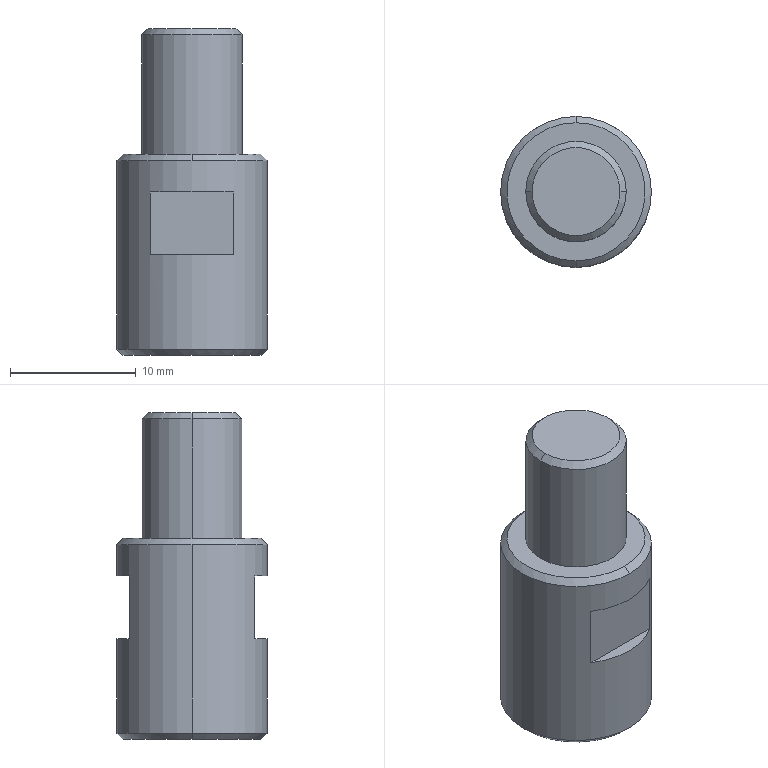Part | STEP file | PN_0019 Locating pin | 1 solid | 19 faces | box 12 x 12 x 26 mm | volume 2255 mm3 | plane 9 | cone 6 | cylinder 4 | commonest cylinder face diameters 8 x2 12 x2
STEP:
#1=CARTESIAN_POINT('',(0.,0.,0.));
#2=DIRECTION('',(0.,0.,1.));
#3=DIRECTION('',(1.,0.,0.));
#4=AXIS2_PLACEMENT_3D('',#1,#2,#3);
#5=CARTESIAN_POINT('',(-3.317,5.,8.));
#6=VERTEX_POINT('',#5);
#7=CARTESIAN_POINT('',(3.317,5.,8.));
#8=VERTEX_POINT('',#7);
#9=CARTESIAN_POINT('',(0.,0.,8.));
#10=DIRECTION('',(0.,0.,-1.));
#11=DIRECTION('',(-1.,0.,0.));
#12=AXIS2_PLACEMENT_3D('',#9,#10,#11);
#13=CIRCLE('',#12,6.);
#14=CARTESIAN_POINT('',(0.,0.,16.));
#15=DIRECTION('',(0.,0.,-1.));
#16=DIRECTION('',(-1.,0.,0.));
#17=AXIS2_PLACEMENT_3D('',#14,#15,#16);
#18=CYLINDRICAL_SURFACE('',#17,6.);
#19=CARTESIAN_POINT('',(0.,8.));
#20=DIRECTION('',(1.,0.));
#21=VECTOR('',#20,1.);
#22=LINE('',#19,#21);
#23=(GEOMETRIC_REPRESENTATION_CONTEXT(2)PARAMETRIC_REPRESENTATION_CONTEXT()REPRESENTATION_CONTEXT('',''));
#24=DEFINITIONAL_REPRESENTATION('',(#22),#23);
#25=PCURVE('',#18,#24);
#26=CARTESIAN_POINT('',(-6.,10.,8.));
#27=DIRECTION('',(0.,0.,-1.));
#28=DIRECTION('',(-1.,0.,0.));
#29=AXIS2_PLACEMENT_3D('',#26,#27,#28);
#30=PLANE('',#29);
#31=CARTESIAN_POINT('',(-6.,-10.));
#32=DIRECTION('',(1.,0.));
#33=AXIS2_PLACEMENT_2D('',#31,#32);
#34=CIRCLE('',#33,6.);
#35=(GEOMETRIC_REPRESENTATION_CONTEXT(2)PARAMETRIC_REPRESENTATION_CONTEXT()REPRESENTATION_CONTEXT('',''));
#36=DEFINITIONAL_REPRESENTATION('',(#34),#35);
#37=PCURVE('',#30,#36);
#38=SURFACE_CURVE('',#13,(#25,#37),.PCURVE_S1.);
#39=EDGE_CURVE('',#6,#8,#38,.T.);
#40=ORIENTED_EDGE('',*,*,#39,.T.);
#41=CARTESIAN_POINT('',(3.317,5.,13.));
#42=VERTEX_POINT('',#41);
#43=CARTESIAN_POINT('',(3.317,5.,16.));
#44=DIRECTION('',(0.,0.,1.));
#45=VECTOR('',#44,1.);
#46=LINE('',#43,#45);
#47=CARTESIAN_POINT('',(2.156,0.));
#48=DIRECTION('',(0.,-1.));
#49=VECTOR('',#48,1.);
#50=LINE('',#47,#49);
#51=(GEOMETRIC_REPRESENTATION_CONTEXT(2)PARAMETRIC_REPRESENTATION_CONTEXT()REPRESENTATION_CONTEXT('',''));
#52=DEFINITIONAL_REPRESENTATION('',(#50),#51);
#53=PCURVE('',#18,#52);
#54=CARTESIAN_POINT('',(-6.,5.,8.));
#55=DIRECTION('',(0.,-1.,0.));
#56=DIRECTION('',(0.,0.,-1.));
#57=AXIS2_PLACEMENT_3D('',#54,#55,#56);
#58=PLANE('',#57);
#59=CARTESIAN_POINT('',(-8.,9.317));
#60=DIRECTION('',(-1.,0.));
#61=VECTOR('',#60,1.);
#62=LINE('',#59,#61);
#63=(GEOMETRIC_REPRESENTATION_CONTEXT(2)PARAMETRIC_REPRESENTATION_CONTEXT()REPRESENTATION_CONTEXT('',''));
#64=DEFINITIONAL_REPRESENTATION('',(#62),#63);
#65=PCURVE('',#58,#64);
#66=SURFACE_CURVE('',#46,(#53,#65),.PCURVE_S1.);
#67=EDGE_CURVE('',#8,#42,#66,.T.);
#68=ORIENTED_EDGE('',*,*,#67,.T.);
#69=CARTESIAN_POINT('',(-3.317,5.,13.));
#70=VERTEX_POINT('',#69);
#71=CARTESIAN_POINT('',(0.,0.,13.));
#72=DIRECTION('',(0.,0.,1.));
#73=DIRECTION('',(-1.,0.,0.));
#74=AXIS2_PLACEMENT_3D('',#71,#72,#73);
#75=CIRCLE('',#74,6.);
#76=CARTESIAN_POINT('',(6.283,3.));
#77=DIRECTION('',(-1.,0.));
#78=VECTOR('',#77,1.);
#79=LINE('',#76,#78);
#80=(GEOMETRIC_REPRESENTATION_CONTEXT(2)PARAMETRIC_REPRESENTATION_CONTEXT()REPRESENTATION_CONTEXT('',''));
#81=DEFINITIONAL_REPRESENTATION('',(#79),#80);
#82=PCURVE('',#18,#81);
#83=CARTESIAN_POINT('',(-6.,10.,13.));
#84=DIRECTION('',(0.,0.,1.));
#85=DIRECTION('',(1.,0.,0.));
#86=AXIS2_PLACEMENT_3D('',#83,#84,#85);
#87=PLANE('',#86);
#88=CARTESIAN_POINT('',(6.,-10.));
#89=DIRECTION('',(-1.,0.));
#90=AXIS2_PLACEMENT_2D('',#88,#89);
#91=CIRCLE('',#90,6.);
#92=(GEOMETRIC_REPRESENTATION_CONTEXT(2)PARAMETRIC_REPRESENTATION_CONTEXT()REPRESENTATION_CONTEXT('',''));
#93=DEFINITIONAL_REPRESENTATION('',(#91),#92);
#94=PCURVE('',#87,#93);
#95=SURFACE_CURVE('',#75,(#82,#94),.PCURVE_S1.);
#96=EDGE_CURVE('',#42,#70,#95,.T.);
#97=ORIENTED_EDGE('',*,*,#96,.T.);
#98=CARTESIAN_POINT('',(-3.317,5.,16.));
#99=DIRECTION('',(0.,0.,-1.));
#100=VECTOR('',#99,1.);
#101=LINE('',#98,#100);
#102=CARTESIAN_POINT('',(0.9851,0.));
#103=DIRECTION('',(0.,1.));
#104=VECTOR('',#103,1.);
#105=LINE('',#102,#104);
#106=(GEOMETRIC_REPRESENTATION_CONTEXT(2)PARAMETRIC_REPRESENTATION_CONTEXT()REPRESENTATION_CONTEXT('',''));
#107=DEFINITIONAL_REPRESENTATION('',(#105),#106);
#108=PCURVE('',#18,#107);
#109=CARTESIAN_POINT('',(-8.,2.683));
#110=DIRECTION('',(1.,0.));
#111=VECTOR('',#110,1.);
#112=LINE('',#109,#111);
#113=(GEOMETRIC_REPRESENTATION_CONTEXT(2)PARAMETRIC_REPRESENTATION_CONTEXT()REPRESENTATION_CONTEXT('',''));
#114=DEFINITIONAL_REPRESENTATION('',(#112),#113);
#115=PCURVE('',#58,#114);
#116=SURFACE_CURVE('',#101,(#108,#115),.PCURVE_S1.);
#117=EDGE_CURVE('',#70,#6,#116,.T.);
#118=ORIENTED_EDGE('',*,*,#117,.T.);
#119=EDGE_LOOP('',(#40,#68,#97,#118));
#120=FACE_BOUND('',#119,.T.);
#121=CARTESIAN_POINT('',(0.,6.,15.5));
#122=VERTEX_POINT('',#121);
#123=CARTESIAN_POINT('',(6.,0.,15.5));
#124=VERTEX_POINT('',#123);
#125=CARTESIAN_POINT('',(0.,0.,15.5));
#126=DIRECTION('',(0.,0.,-1.));
#127=DIRECTION('',(-1.,0.,0.));
#128=AXIS2_PLACEMENT_3D('',#125,#126,#127);
#129=CIRCLE('',#128,6.);
#130=CARTESIAN_POINT('',(0.,0.5));
#131=DIRECTION('',(1.,0.));
#132=VECTOR('',#131,1.);
#133=LINE('',#130,#132);
#134=(GEOMETRIC_REPRESENTATION_CONTEXT(2)PARAMETRIC_REPRESENTATION_CONTEXT()REPRESENTATION_CONTEXT('',''));
#135=DEFINITIONAL_REPRESENTATION('',(#133),#134);
#136=PCURVE('',#18,#135);
#137=CARTESIAN_POINT('',(0.,0.,15.5));
#138=DIRECTION('',(0.,0.,-1.));
#139=DIRECTION('',(0.,1.,0.));
#140=AXIS2_PLACEMENT_3D('',#137,#138,#139);
#141=CONICAL_SURFACE('',#140,6.,0.7854);
#142=CARTESIAN_POINT('',(-1.571,0.));
#143=DIRECTION('',(1.,0.));
#144=VECTOR('',#143,1.);
#145=LINE('',#142,#144);
#146=(GEOMETRIC_REPRESENTATION_CONTEXT(2)PARAMETRIC_REPRESENTATION_CONTEXT()REPRESENTATION_CONTEXT('',''));
#147=DEFINITIONAL_REPRESENTATION('',(#145),#146);
#148=PCURVE('',#141,#147);
#149=SURFACE_CURVE('',#129,(#136,#148),.PCURVE_S1.);
#150=EDGE_CURVE('',#122,#124,#149,.T.);
#151=ORIENTED_EDGE('',*,*,#150,.T.);
#152=CARTESIAN_POINT('',(6.,0.,0.5));
#153=VERTEX_POINT('',#152);
#154=CARTESIAN_POINT('',(6.,0.,16.));
#155=DIRECTION('',(0.,0.,-1.));
#156=VECTOR('',#155,1.);
#157=LINE('',#154,#156);
#158=CARTESIAN_POINT('',(3.142,0.));
#159=DIRECTION('',(0.,1.));
#160=VECTOR('',#159,1.);
#161=LINE('',#158,#160);
#162=(GEOMETRIC_REPRESENTATION_CONTEXT(2)PARAMETRIC_REPRESENTATION_CONTEXT()REPRESENTATION_CONTEXT('',''));
#163=DEFINITIONAL_REPRESENTATION('',(#161),#162);
#164=PCURVE('',#18,#163);
#165=CARTESIAN_POINT('',(0.,0.,16.));
#166=DIRECTION('',(0.,0.,-1.));
#167=DIRECTION('',(-1.,0.,0.));
#168=AXIS2_PLACEMENT_3D('',#165,#166,#167);
#169=CYLINDRICAL_SURFACE('',#168,6.);
#170=CARTESIAN_POINT('',(3.142,0.));
#171=DIRECTION('',(0.,1.));
#172=VECTOR('',#171,1.);
#173=LINE('',#170,#172);
#174=(GEOMETRIC_REPRESENTATION_CONTEXT(2)PARAMETRIC_REPRESENTATION_CONTEXT()REPRESENTATION_CONTEXT('',''));
#175=DEFINITIONAL_REPRESENTATION('',(#173),#174);
#176=PCURVE('',#169,#175);
#177=SURFACE_CURVE('',#157,(#164,#176),.PCURVE_S1.);
#178=EDGE_CURVE('',#124,#153,#177,.T.);
#179=ORIENTED_EDGE('',*,*,#178,.T.);
#180=CARTESIAN_POINT('',(-6.,0.,0.5));
#181=VERTEX_POINT('',#180);
#182=CARTESIAN_POINT('',(0.,0.,0.5));
#183=DIRECTION('',(0.,0.,1.));
#184=DIRECTION('',(-1.,0.,0.));
#185=AXIS2_PLACEMENT_3D('',#182,#183,#184);
#186=CIRCLE('',#185,6.);
#187=CARTESIAN_POINT('',(6.283,15.5));
#188=DIRECTION('',(-1.,0.));
#189=VECTOR('',#188,1.);
#190=LINE('',#187,#189);
#191=(GEOMETRIC_REPRESENTATION_CONTEXT(2)PARAMETRIC_REPRESENTATION_CONTEXT()REPRESENTATION_CONTEXT('',''));
#192=DEFINITIONAL_REPRESENTATION('',(#190),#191);
#193=PCURVE('',#18,#192);
#194=CARTESIAN_POINT('',(0.,0.,0.5));
#195=DIRECTION('',(0.,0.,1.));
#196=DIRECTION('',(1.,0.,0.));
#197=AXIS2_PLACEMENT_3D('',#194,#195,#196);
#198=CONICAL_SURFACE('',#197,6.,0.7854);
#199=CARTESIAN_POINT('',(-3.142,0.));
#200=DIRECTION('',(1.,0.));
#201=VECTOR('',#200,1.);
#202=LINE('',#199,#201);
#203=(GEOMETRIC_REPRESENTATION_CONTEXT(2)PARAMETRIC_REPRESENTATION_CONTEXT()REPRESENTATION_CONTEXT('',''));
#204=DEFINITIONAL_REPRESENTATION('',(#202),#203);
#205=PCURVE('',#198,#204);
#206=SURFACE_CURVE('',#186,(#193,#205),.PCURVE_S1.);
#207=EDGE_CURVE('',#153,#181,#206,.T.);
#208=ORIENTED_EDGE('',*,*,#207,.T.);
#209=CARTESIAN_POINT('',(-6.,0.,15.5));
#210=VERTEX_POINT('',#209);
#211=CARTESIAN_POINT('',(-6.,0.,16.));
#212=DIRECTION('',(0.,0.,-1.));
#213=VECTOR('',#212,1.);
#214=LINE('',#211,#213);
#215=CARTESIAN_POINT('',(0.,0.));
#216=DIRECTION('',(0.,1.));
#217=VECTOR('',#216,1.);
#218=LINE('',#215,#217);
#219=(GEOMETRIC_REPRESENTATION_CONTEXT(2)PARAMETRIC_REPRESENTATION_CONTEXT()REPRESENTATION_CONTEXT('',''));
#220=DEFINITIONAL_REPRESENTATION('',(#218),#219);
#221=PCURVE('',#18,#220);
#222=CARTESIAN_POINT('',(6.283,0.));
#223=DIRECTION('',(0.,1.));
#224=VECTOR('',#223,1.);
#225=LINE('',#222,#224);
#226=(GEOMETRIC_REPRESENTATION_CONTEXT(2)PARAMETRIC_REPRESENTATION_CONTEXT()REPRESENTATION_CONTEXT('',''));
#227=DEFINITIONAL_REPRESENTATION('',(#225),#226);
#228=PCURVE('',#169,#227);
#229=SURFACE_CURVE('',#214,(#221,#228),.PCURVE_S1.);
#230=EDGE_CURVE('',#210,#181,#229,.T.);
#231=ORIENTED_EDGE('',*,*,#230,.F.);
#232=CARTESIAN_POINT('',(0.,0.,15.5));
#233=DIRECTION('',(0.,0.,-1.));
#234=DIRECTION('',(-1.,0.,0.));
#235=AXIS2_PLACEMENT_3D('',#232,#233,#234);
#236=CIRCLE('',#235,6.);
#237=CARTESIAN_POINT('',(0.,0.5));
#238=DIRECTION('',(1.,0.));
#239=VECTOR('',#238,1.);
#240=LINE('',#237,#239);
#241=(GEOMETRIC_REPRESENTATION_CONTEXT(2)PARAMETRIC_REPRESENTATION_CONTEXT()REPRESENTATION_CONTEXT('',''));
#242=DEFINITIONAL_REPRESENTATION('',(#240),#241);
#243=PCURVE('',#18,#242);
#244=CARTESIAN_POINT('',(0.,0.,15.5));
#245=DIRECTION('',(0.,0.,-1.));
#246=DIRECTION('',(0.,1.,0.));
#247=AXIS2_PLACEMENT_3D('',#244,#245,#246);
#248=CONICAL_SURFACE('',#247,6.,0.7854);
#249=CARTESIAN_POINT('',(4.712,0.));
#250=DIRECTION('',(1.,0.));
#251=VECTOR('',#250,1.);
#252=LINE('',#249,#251);
#253=(GEOMETRIC_REPRESENTATION_CONTEXT(2)PARAMETRIC_REPRESENTATION_CONTEXT()REPRESENTATION_CONTEXT('',''));
#254=DEFINITIONAL_REPRESENTATION('',(#252),#253);
#255=PCURVE('',#248,#254);
#256=SURFACE_CURVE('',#236,(#243,#255),.PCURVE_S1.);
#257=EDGE_CURVE('',#210,#122,#256,.T.);
#258=ORIENTED_EDGE('',*,*,#257,.T.);
#259=EDGE_LOOP('',(#151,#179,#208,#231,#258));
#260=FACE_BOUND('',#259,.T.);
#261=ADVANCED_FACE('',(#120,#260),#18,.T.);
#262=CARTESIAN_POINT('',(5.5,0.,0.));
#263=VERTEX_POINT('',#262);
#264=CARTESIAN_POINT('',(-5.5,0.,0.));
#265=VERTEX_POINT('',#264);
#266=CARTESIAN_POINT('',(0.,0.,0.));
#267=DIRECTION('',(0.,0.,1.));
#268=DIRECTION('',(1.,0.,0.));
#269=AXIS2_PLACEMENT_3D('',#266,#267,#268);
#270=CIRCLE('',#269,5.5);
#271=CARTESIAN_POINT('',(0.,-0.5));
#272=DIRECTION('',(1.,0.));
#273=VECTOR('',#272,1.);
#274=LINE('',#271,#273);
#275=(GEOMETRIC_REPRESENTATION_CONTEXT(2)PARAMETRIC_REPRESENTATION_CONTEXT()REPRESENTATION_CONTEXT('',''));
#276=DEFINITIONAL_REPRESENTATION('',(#274),#275);
#277=PCURVE('',#198,#276);
#278=CARTESIAN_POINT('',(0.,0.,0.));
#279=DIRECTION('',(0.,0.,1.));
#280=DIRECTION('',(1.,0.,0.));
#281=AXIS2_PLACEMENT_3D('',#278,#279,#280);
#282=PLANE('',#281);
#283=CARTESIAN_POINT('',(0.,0.));
#284=DIRECTION('',(1.,0.));
#285=AXIS2_PLACEMENT_2D('',#283,#284);
#286=CIRCLE('',#285,5.5);
#287=(GEOMETRIC_REPRESENTATION_CONTEXT(2)PARAMETRIC_REPRESENTATION_CONTEXT()REPRESENTATION_CONTEXT('',''));
#288=DEFINITIONAL_REPRESENTATION('',(#286),#287);
#289=PCURVE('',#282,#288);
#290=SURFACE_CURVE('',#270,(#277,#289),.PCURVE_S1.);
#291=EDGE_CURVE('',#263,#265,#290,.T.);
#292=ORIENTED_EDGE('',*,*,#291,.T.);
#293=CARTESIAN_POINT('',(-6.,0.,0.5));
#294=DIRECTION('',(-0.7071,0.,0.7071));
#295=VECTOR('',#294,1.);
#296=LINE('',#293,#295);
#297=CARTESIAN_POINT('',(3.142,0.));
#298=DIRECTION('',(0.,1.));
#299=VECTOR('',#298,1.);
#300=LINE('',#297,#299);
#301=(GEOMETRIC_REPRESENTATION_CONTEXT(2)PARAMETRIC_REPRESENTATION_CONTEXT()REPRESENTATION_CONTEXT('',''));
#302=DEFINITIONAL_REPRESENTATION('',(#300),#301);
#303=PCURVE('',#198,#302);
#304=CARTESIAN_POINT('',(0.,0.,0.5));
#305=DIRECTION('',(0.,0.,1.));
#306=DIRECTION('',(1.,0.,0.));
#307=AXIS2_PLACEMENT_3D('',#304,#305,#306);
#308=CONICAL_SURFACE('',#307,6.,0.7854);
#309=CARTESIAN_POINT('',(3.142,0.));
#310=DIRECTION('',(0.,1.));
#311=VECTOR('',#310,1.);
#312=LINE('',#309,#311);
#313=(GEOMETRIC_REPRESENTATION_CONTEXT(2)PARAMETRIC_REPRESENTATION_CONTEXT()REPRESENTATION_CONTEXT('',''));
#314=DEFINITIONAL_REPRESENTATION('',(#312),#313);
#315=PCURVE('',#308,#314);
#316=SURFACE_CURVE('',#296,(#303,#315),.PCURVE_S1.);
#317=EDGE_CURVE('',#265,#181,#316,.T.);
#318=ORIENTED_EDGE('',*,*,#317,.T.);
#319=ORIENTED_EDGE('',*,*,#207,.F.);
#320=CARTESIAN_POINT('',(6.,0.,0.5));
#321=DIRECTION('',(0.7071,0.,0.7071));
#322=VECTOR('',#321,1.);
#323=LINE('',#320,#322);
#324=CARTESIAN_POINT('',(0.,0.));
#325=DIRECTION('',(0.,1.));
#326=VECTOR('',#325,1.);
#327=LINE('',#324,#326);
#328=(GEOMETRIC_REPRESENTATION_CONTEXT(2)PARAMETRIC_REPRESENTATION_CONTEXT()REPRESENTATION_CONTEXT('',''));
#329=DEFINITIONAL_REPRESENTATION('',(#327),#328);
#330=PCURVE('',#198,#329);
#331=CARTESIAN_POINT('',(6.283,0.));
#332=DIRECTION('',(0.,1.));
#333=VECTOR('',#332,1.);
#334=LINE('',#331,#333);
#335=(GEOMETRIC_REPRESENTATION_CONTEXT(2)PARAMETRIC_REPRESENTATION_CONTEXT()REPRESENTATION_CONTEXT('',''));
#336=DEFINITIONAL_REPRESENTATION('',(#334),#335);
#337=PCURVE('',#308,#336);
#338=SURFACE_CURVE('',#323,(#330,#337),.PCURVE_S1.);
#339=EDGE_CURVE('',#263,#153,#338,.T.);
#340=ORIENTED_EDGE('',*,*,#339,.F.);
#341=EDGE_LOOP('',(#292,#318,#319,#340));
#342=FACE_BOUND('',#341,.T.);
#343=ADVANCED_FACE('',(#342),#198,.T.);
#344=CARTESIAN_POINT('',(0.,5.5,16.));
#345=VERTEX_POINT('',#344);
#346=CARTESIAN_POINT('',(0.,-5.5,16.));
#347=VERTEX_POINT('',#346);
#348=CARTESIAN_POINT('',(0.,0.,16.));
#349=DIRECTION('',(0.,0.,-1.));
#350=DIRECTION('',(0.,1.,0.));
#351=AXIS2_PLACEMENT_3D('',#348,#349,#350);
#352=CIRCLE('',#351,5.5);
#353=CARTESIAN_POINT('',(0.,-0.5));
#354=DIRECTION('',(1.,0.));
#355=VECTOR('',#354,1.);
#356=LINE('',#353,#355);
#357=(GEOMETRIC_REPRESENTATION_CONTEXT(2)PARAMETRIC_REPRESENTATION_CONTEXT()REPRESENTATION_CONTEXT('',''));
#358=DEFINITIONAL_REPRESENTATION('',(#356),#357);
#359=PCURVE('',#141,#358);
#360=CARTESIAN_POINT('',(0.,0.,16.));
#361=DIRECTION('',(0.,0.,1.));
#362=DIRECTION('',(1.,0.,0.));
#363=AXIS2_PLACEMENT_3D('',#360,#361,#362);
#364=PLANE('',#363);
#365=CARTESIAN_POINT('',(0.,5.5));
#366=CARTESIAN_POINT('',(9.526,5.5));
#367=CARTESIAN_POINT('',(4.763,-2.75));
#368=CARTESIAN_POINT('',(0.,-11.));
#369=CARTESIAN_POINT('',(-4.763,-2.75));
#370=CARTESIAN_POINT('',(-9.526,5.5));
#371=CARTESIAN_POINT('',(0.,5.5));
#372=(BOUNDED_CURVE()B_SPLINE_CURVE(2,(#365,#366,#367,#368,#369,#370,#371),.UNSPECIFIED.,.T.,.F.)B_SPLINE_CURVE_WITH_KNOTS((1,2,2,2,2,1),(-2.094,0.,2.094,4.189,6.283,8.378),.UNSPECIFIED.)CURVE()GEOMETRIC_REPRESENTATION_ITEM()RATIONAL_B_SPLINE_CURVE((1.,0.5,1.,0.5,1.,0.5,1.))REPRESENTATION_ITEM(''));
#373=(GEOMETRIC_REPRESENTATION_CONTEXT(2)PARAMETRIC_REPRESENTATION_CONTEXT()REPRESENTATION_CONTEXT('',''));
#374=DEFINITIONAL_REPRESENTATION('',(#372),#373);
#375=PCURVE('',#364,#374);
#376=SURFACE_CURVE('',#352,(#359,#375),.PCURVE_S1.);
#377=EDGE_CURVE('',#345,#347,#376,.T.);
#378=ORIENTED_EDGE('',*,*,#377,.T.);
#379=CARTESIAN_POINT('',(0.,-6.,15.5));
#380=VERTEX_POINT('',#379);
#381=CARTESIAN_POINT('',(0.,-6.,15.5));
#382=DIRECTION('',(0.,-0.7071,-0.7071));
#383=VECTOR('',#382,1.);
#384=LINE('',#381,#383);
#385=CARTESIAN_POINT('',(3.142,0.));
#386=DIRECTION('',(0.,1.));
#387=VECTOR('',#386,1.);
#388=LINE('',#385,#387);
#389=(GEOMETRIC_REPRESENTATION_CONTEXT(2)PARAMETRIC_REPRESENTATION_CONTEXT()REPRESENTATION_CONTEXT('',''));
#390=DEFINITIONAL_REPRESENTATION('',(#388),#389);
#391=PCURVE('',#141,#390);
#392=CARTESIAN_POINT('',(3.142,0.));
#393=DIRECTION('',(0.,1.));
#394=VECTOR('',#393,1.);
#395=LINE('',#392,#394);
#396=(GEOMETRIC_REPRESENTATION_CONTEXT(2)PARAMETRIC_REPRESENTATION_CONTEXT()REPRESENTATION_CONTEXT('',''));
#397=DEFINITIONAL_REPRESENTATION('',(#395),#396);
#398=PCURVE('',#248,#397);
#399=SURFACE_CURVE('',#384,(#391,#398),.PCURVE_S1.);
#400=EDGE_CURVE('',#347,#380,#399,.T.);
#401=ORIENTED_EDGE('',*,*,#400,.T.);
#402=CARTESIAN_POINT('',(0.,0.,15.5));
#403=DIRECTION('',(0.,0.,-1.));
#404=DIRECTION('',(-1.,0.,0.));
#405=AXIS2_PLACEMENT_3D('',#402,#403,#404);
#406=CIRCLE('',#405,6.);
#407=CARTESIAN_POINT('',(-1.571,0.));
#408=DIRECTION('',(1.,0.));
#409=VECTOR('',#408,1.);
#410=LINE('',#407,#409);
#411=(GEOMETRIC_REPRESENTATION_CONTEXT(2)PARAMETRIC_REPRESENTATION_CONTEXT()REPRESENTATION_CONTEXT('',''));
#412=DEFINITIONAL_REPRESENTATION('',(#410),#411);
#413=PCURVE('',#141,#412);
#414=CARTESIAN_POINT('',(0.,0.5));
#415=DIRECTION('',(1.,0.));
#416=VECTOR('',#415,1.);
#417=LINE('',#414,#416);
#418=(GEOMETRIC_REPRESENTATION_CONTEXT(2)PARAMETRIC_REPRESENTATION_CONTEXT()REPRESENTATION_CONTEXT('',''));
#419=DEFINITIONAL_REPRESENTATION('',(#417),#418);
#420=PCURVE('',#169,#419);
#421=SURFACE_CURVE('',#406,(#413,#420),.PCURVE_S1.);
#422=EDGE_CURVE('',#124,#380,#421,.T.);
#423=ORIENTED_EDGE('',*,*,#422,.F.);
#424=ORIENTED_EDGE('',*,*,#150,.F.);
#425=CARTESIAN_POINT('',(0.,6.,15.5));
#426=DIRECTION('',(0.,0.7071,-0.7071));
#427=VECTOR('',#426,1.);
#428=LINE('',#425,#427);
#429=CARTESIAN_POINT('',(0.,0.));
#430=DIRECTION('',(0.,1.));
#431=VECTOR('',#430,1.);
#432=LINE('',#429,#431);
#433=(GEOMETRIC_REPRESENTATION_CONTEXT(2)PARAMETRIC_REPRESENTATION_CONTEXT()REPRESENTATION_CONTEXT('',''));
#434=DEFINITIONAL_REPRESENTATION('',(#432),#433);
#435=PCURVE('',#141,#434);
#436=CARTESIAN_POINT('',(6.283,0.));
#437=DIRECTION('',(0.,1.));
#438=VECTOR('',#437,1.);
#439=LINE('',#436,#438);
#440=(GEOMETRIC_REPRESENTATION_CONTEXT(2)PARAMETRIC_REPRESENTATION_CONTEXT()REPRESENTATION_CONTEXT('',''));
#441=DEFINITIONAL_REPRESENTATION('',(#439),#440);
#442=PCURVE('',#248,#441);
#443=SURFACE_CURVE('',#428,(#435,#442),.PCURVE_S1.);
#444=EDGE_CURVE('',#345,#122,#443,.T.);
#445=ORIENTED_EDGE('',*,*,#444,.F.);
#446=EDGE_LOOP('',(#378,#401,#423,#424,#445));
#447=FACE_BOUND('',#446,.T.);
#448=ADVANCED_FACE('',(#447),#141,.T.);
#449=CARTESIAN_POINT('',(-4.,0.,25.5));
#450=VERTEX_POINT('',#449);
#451=CARTESIAN_POINT('',(4.,0.,25.5));
#452=VERTEX_POINT('',#451);
#453=CARTESIAN_POINT('',(0.,0.,25.5));
#454=DIRECTION('',(0.,0.,-1.));
#455=DIRECTION('',(-1.,0.,0.));
#456=AXIS2_PLACEMENT_3D('',#453,#454,#455);
#457=CIRCLE('',#456,4.);
#458=CARTESIAN_POINT('',(0.,0.,26.));
#459=DIRECTION('',(0.,0.,-1.));
#460=DIRECTION('',(-1.,0.,0.));
#461=AXIS2_PLACEMENT_3D('',#458,#459,#460);
#462=CYLINDRICAL_SURFACE('',#461,4.);
#463=CARTESIAN_POINT('',(0.,0.5));
#464=DIRECTION('',(1.,0.));
#465=VECTOR('',#464,1.);
#466=LINE('',#463,#465);
#467=(GEOMETRIC_REPRESENTATION_CONTEXT(2)PARAMETRIC_REPRESENTATION_CONTEXT()REPRESENTATION_CONTEXT('',''));
#468=DEFINITIONAL_REPRESENTATION('',(#466),#467);
#469=PCURVE('',#462,#468);
#470=CARTESIAN_POINT('',(0.,0.,25.5));
#471=DIRECTION('',(0.,0.,-1.));
#472=DIRECTION('',(-1.,0.,0.));
#473=AXIS2_PLACEMENT_3D('',#470,#471,#472);
#474=CONICAL_SURFACE('',#473,4.,0.7854);
#475=CARTESIAN_POINT('',(0.,0.));
#476=DIRECTION('',(1.,0.));
#477=VECTOR('',#476,1.);
#478=LINE('',#475,#477);
#479=(GEOMETRIC_REPRESENTATION_CONTEXT(2)PARAMETRIC_REPRESENTATION_CONTEXT()REPRESENTATION_CONTEXT('',''));
#480=DEFINITIONAL_REPRESENTATION('',(#478),#479);
#481=PCURVE('',#474,#480);
#482=SURFACE_CURVE('',#457,(#469,#481),.PCURVE_S1.);
#483=EDGE_CURVE('',#450,#452,#482,.T.);
#484=ORIENTED_EDGE('',*,*,#483,.T.);
#485=CARTESIAN_POINT('',(4.,0.,16.));
#486=VERTEX_POINT('',#485);
#487=CARTESIAN_POINT('',(4.,0.,26.));
#488=DIRECTION('',(0.,0.,-1.));
#489=VECTOR('',#488,1.);
#490=LINE('',#487,#489);
#491=CARTESIAN_POINT('',(3.142,0.));
#492=DIRECTION('',(0.,1.));
#493=VECTOR('',#492,1.);
#494=LINE('',#491,#493);
#495=(GEOMETRIC_REPRESENTATION_CONTEXT(2)PARAMETRIC_REPRESENTATION_CONTEXT()REPRESENTATION_CONTEXT('',''));
#496=DEFINITIONAL_REPRESENTATION('',(#494),#495);
#497=PCURVE('',#462,#496);
#498=CARTESIAN_POINT('',(0.,0.,26.));
#499=DIRECTION('',(0.,0.,-1.));
#500=DIRECTION('',(-1.,0.,0.));
#501=AXIS2_PLACEMENT_3D('',#498,#499,#500);
#502=CYLINDRICAL_SURFACE('',#501,4.);
#503=CARTESIAN_POINT('',(3.142,0.));
#504=DIRECTION('',(0.,1.));
#505=VECTOR('',#504,1.);
#506=LINE('',#503,#505);
#507=(GEOMETRIC_REPRESENTATION_CONTEXT(2)PARAMETRIC_REPRESENTATION_CONTEXT()REPRESENTATION_CONTEXT('',''));
#508=DEFINITIONAL_REPRESENTATION('',(#506),#507);
#509=PCURVE('',#502,#508);
#510=SURFACE_CURVE('',#490,(#497,#509),.PCURVE_S1.);
#511=EDGE_CURVE('',#452,#486,#510,.T.);
#512=ORIENTED_EDGE('',*,*,#511,.T.);
#513=CARTESIAN_POINT('',(-4.,0.,16.));
#514=VERTEX_POINT('',#513);
#515=CARTESIAN_POINT('',(0.,0.,16.));
#516=DIRECTION('',(0.,0.,-1.));
#517=DIRECTION('',(-1.,0.,0.));
#518=AXIS2_PLACEMENT_3D('',#515,#516,#517);
#519=CIRCLE('',#518,4.);
#520=CARTESIAN_POINT('',(0.,10.));
#521=DIRECTION('',(1.,0.));
#522=VECTOR('',#521,1.);
#523=LINE('',#520,#522);
#524=(GEOMETRIC_REPRESENTATION_CONTEXT(2)PARAMETRIC_REPRESENTATION_CONTEXT()REPRESENTATION_CONTEXT('',''));
#525=DEFINITIONAL_REPRESENTATION('',(#523),#524);
#526=PCURVE('',#462,#525);
#527=CARTESIAN_POINT('',(-4.,0.));
#528=CARTESIAN_POINT('',(-4.,6.928));
#529=CARTESIAN_POINT('',(2.,3.464));
#530=CARTESIAN_POINT('',(8.,0.));
#531=CARTESIAN_POINT('',(2.,-3.464));
#532=CARTESIAN_POINT('',(-4.,-6.928));
#533=CARTESIAN_POINT('',(-4.,0.));
#534=(BOUNDED_CURVE()B_SPLINE_CURVE(2,(#527,#528,#529,#530,#531,#532,#533),.UNSPECIFIED.,.T.,.F.)B_SPLINE_CURVE_WITH_KNOTS((1,2,2,2,2,1),(-2.094,0.,2.094,4.189,6.283,8.378),.UNSPECIFIED.)CURVE()GEOMETRIC_REPRESENTATION_ITEM()RATIONAL_B_SPLINE_CURVE((1.,0.5,1.,0.5,1.,0.5,1.))REPRESENTATION_ITEM(''));
#535=(GEOMETRIC_REPRESENTATION_CONTEXT(2)PARAMETRIC_REPRESENTATION_CONTEXT()REPRESENTATION_CONTEXT('',''));
#536=DEFINITIONAL_REPRESENTATION('',(#534),#535);
#537=PCURVE('',#364,#536);
#538=SURFACE_CURVE('',#519,(#526,#537),.PCURVE_S1.);
#539=EDGE_CURVE('',#514,#486,#538,.T.);
#540=ORIENTED_EDGE('',*,*,#539,.F.);
#541=CARTESIAN_POINT('',(-4.,0.,26.));
#542=DIRECTION('',(0.,0.,-1.));
#543=VECTOR('',#542,1.);
#544=LINE('',#541,#543);
#545=CARTESIAN_POINT('',(0.,0.));
#546=DIRECTION('',(0.,1.));
#547=VECTOR('',#546,1.);
#548=LINE('',#545,#547);
#549=(GEOMETRIC_REPRESENTATION_CONTEXT(2)PARAMETRIC_REPRESENTATION_CONTEXT()REPRESENTATION_CONTEXT('',''));
#550=DEFINITIONAL_REPRESENTATION('',(#548),#549);
#551=PCURVE('',#462,#550);
#552=CARTESIAN_POINT('',(6.283,0.));
#553=DIRECTION('',(0.,1.));
#554=VECTOR('',#553,1.);
#555=LINE('',#552,#554);
#556=(GEOMETRIC_REPRESENTATION_CONTEXT(2)PARAMETRIC_REPRESENTATION_CONTEXT()REPRESENTATION_CONTEXT('',''));
#557=DEFINITIONAL_REPRESENTATION('',(#555),#556);
#558=PCURVE('',#502,#557);
#559=SURFACE_CURVE('',#544,(#551,#558),.PCURVE_S1.);
#560=EDGE_CURVE('',#450,#514,#559,.T.);
#561=ORIENTED_EDGE('',*,*,#560,.F.);
#562=EDGE_LOOP('',(#484,#512,#540,#561));
#563=FACE_BOUND('',#562,.T.);
#564=ADVANCED_FACE('',(#563),#462,.T.);
#565=CARTESIAN_POINT('',(-3.5,0.,26.));
#566=VERTEX_POINT('',#565);
#567=CARTESIAN_POINT('',(3.5,0.,26.));
#568=VERTEX_POINT('',#567);
#569=CARTESIAN_POINT('',(0.,0.,26.));
#570=DIRECTION('',(0.,0.,-1.));
#571=DIRECTION('',(-1.,0.,0.));
#572=AXIS2_PLACEMENT_3D('',#569,#570,#571);
#573=CIRCLE('',#572,3.5);
#574=CARTESIAN_POINT('',(0.,-0.5));
#575=DIRECTION('',(1.,0.));
#576=VECTOR('',#575,1.);
#577=LINE('',#574,#576);
#578=(GEOMETRIC_REPRESENTATION_CONTEXT(2)PARAMETRIC_REPRESENTATION_CONTEXT()REPRESENTATION_CONTEXT('',''));
#579=DEFINITIONAL_REPRESENTATION('',(#577),#578);
#580=PCURVE('',#474,#579);
#581=CARTESIAN_POINT('',(0.,0.,26.));
#582=DIRECTION('',(0.,0.,1.));
#583=DIRECTION('',(1.,0.,0.));
#584=AXIS2_PLACEMENT_3D('',#581,#582,#583);
#585=PLANE('',#584);
#586=CARTESIAN_POINT('',(-3.5,0.));
#587=CARTESIAN_POINT('',(-3.5,6.062));
#588=CARTESIAN_POINT('',(1.75,3.031));
#589=CARTESIAN_POINT('',(7.,0.));
#590=CARTESIAN_POINT('',(1.75,-3.031));
#591=CARTESIAN_POINT('',(-3.5,-6.062));
#592=CARTESIAN_POINT('',(-3.5,0.));
#593=(BOUNDED_CURVE()B_SPLINE_CURVE(2,(#586,#587,#588,#589,#590,#591,#592),.UNSPECIFIED.,.T.,.F.)B_SPLINE_CURVE_WITH_KNOTS((1,2,2,2,2,1),(-2.094,0.,2.094,4.189,6.283,8.378),.UNSPECIFIED.)CURVE()GEOMETRIC_REPRESENTATION_ITEM()RATIONAL_B_SPLINE_CURVE((1.,0.5,1.,0.5,1.,0.5,1.))REPRESENTATION_ITEM(''));
#594=(GEOMETRIC_REPRESENTATION_CONTEXT(2)PARAMETRIC_REPRESENTATION_CONTEXT()REPRESENTATION_CONTEXT('',''));
#595=DEFINITIONAL_REPRESENTATION('',(#593),#594);
#596=PCURVE('',#585,#595);
#597=SURFACE_CURVE('',#573,(#580,#596),.PCURVE_S1.);
#598=EDGE_CURVE('',#566,#568,#597,.T.);
#599=ORIENTED_EDGE('',*,*,#598,.T.);
#600=CARTESIAN_POINT('',(4.,0.,25.5));
#601=DIRECTION('',(0.7071,0.,-0.7071));
#602=VECTOR('',#601,1.);
#603=LINE('',#600,#602);
#604=CARTESIAN_POINT('',(3.142,0.));
#605=DIRECTION('',(0.,1.));
#606=VECTOR('',#605,1.);
#607=LINE('',#604,#606);
#608=(GEOMETRIC_REPRESENTATION_CONTEXT(2)PARAMETRIC_REPRESENTATION_CONTEXT()REPRESENTATION_CONTEXT('',''));
#609=DEFINITIONAL_REPRESENTATION('',(#607),#608);
#610=PCURVE('',#474,#609);
#611=CARTESIAN_POINT('',(0.,0.,25.5));
#612=DIRECTION('',(0.,0.,-1.));
#613=DIRECTION('',(-1.,0.,0.));
#614=AXIS2_PLACEMENT_3D('',#611,#612,#613);
#615=CONICAL_SURFACE('',#614,4.,0.7854);
#616=CARTESIAN_POINT('',(3.142,0.));
#617=DIRECTION('',(0.,1.));
#618=VECTOR('',#617,1.);
#619=LINE('',#616,#618);
#620=(GEOMETRIC_REPRESENTATION_CONTEXT(2)PARAMETRIC_REPRESENTATION_CONTEXT()REPRESENTATION_CONTEXT('',''));
#621=DEFINITIONAL_REPRESENTATION('',(#619),#620);
#622=PCURVE('',#615,#621);
#623=SURFACE_CURVE('',#603,(#610,#622),.PCURVE_S1.);
#624=EDGE_CURVE('',#568,#452,#623,.T.);
#625=ORIENTED_EDGE('',*,*,#624,.T.);
#626=ORIENTED_EDGE('',*,*,#483,.F.);
#627=CARTESIAN_POINT('',(-4.,0.,25.5));
#628=DIRECTION('',(-0.7071,0.,-0.7071));
#629=VECTOR('',#628,1.);
#630=LINE('',#627,#629);
#631=CARTESIAN_POINT('',(0.,0.));
#632=DIRECTION('',(0.,1.));
#633=VECTOR('',#632,1.);
#634=LINE('',#631,#633);
#635=(GEOMETRIC_REPRESENTATION_CONTEXT(2)PARAMETRIC_REPRESENTATION_CONTEXT()REPRESENTATION_CONTEXT('',''));
#636=DEFINITIONAL_REPRESENTATION('',(#634),#635);
#637=PCURVE('',#474,#636);
#638=CARTESIAN_POINT('',(6.283,0.));
#639=DIRECTION('',(0.,1.));
#640=VECTOR('',#639,1.);
#641=LINE('',#638,#640);
#642=(GEOMETRIC_REPRESENTATION_CONTEXT(2)PARAMETRIC_REPRESENTATION_CONTEXT()REPRESENTATION_CONTEXT('',''));
#643=DEFINITIONAL_REPRESENTATION('',(#641),#642);
#644=PCURVE('',#615,#643);
#645=SURFACE_CURVE('',#630,(#637,#644),.PCURVE_S1.);
#646=EDGE_CURVE('',#566,#450,#645,.T.);
#647=ORIENTED_EDGE('',*,*,#646,.F.);
#648=EDGE_LOOP('',(#599,#625,#626,#647));
#649=FACE_BOUND('',#648,.T.);
#650=ADVANCED_FACE('',(#649),#474,.T.);
#651=ORIENTED_EDGE('',*,*,#178,.F.);
#652=ORIENTED_EDGE('',*,*,#422,.T.);
#653=CARTESIAN_POINT('',(0.,0.,15.5));
#654=DIRECTION('',(0.,0.,-1.));
#655=DIRECTION('',(-1.,0.,0.));
#656=AXIS2_PLACEMENT_3D('',#653,#654,#655);
#657=CIRCLE('',#656,6.);
#658=CARTESIAN_POINT('',(0.,0.5));
#659=DIRECTION('',(1.,0.));
#660=VECTOR('',#659,1.);
#661=LINE('',#658,#660);
#662=(GEOMETRIC_REPRESENTATION_CONTEXT(2)PARAMETRIC_REPRESENTATION_CONTEXT()REPRESENTATION_CONTEXT('',''));
#663=DEFINITIONAL_REPRESENTATION('',(#661),#662);
#664=PCURVE('',#169,#663);
#665=CARTESIAN_POINT('',(-1.571,0.));
#666=DIRECTION('',(1.,0.));
#667=VECTOR('',#666,1.);
#668=LINE('',#665,#667);
#669=(GEOMETRIC_REPRESENTATION_CONTEXT(2)PARAMETRIC_REPRESENTATION_CONTEXT()REPRESENTATION_CONTEXT('',''));
#670=DEFINITIONAL_REPRESENTATION('',(#668),#669);
#671=PCURVE('',#248,#670);
#672=SURFACE_CURVE('',#657,(#664,#671),.PCURVE_S1.);
#673=EDGE_CURVE('',#380,#210,#672,.T.);
#674=ORIENTED_EDGE('',*,*,#673,.T.);
#675=ORIENTED_EDGE('',*,*,#230,.T.);
#676=CARTESIAN_POINT('',(0.,0.,0.5));
#677=DIRECTION('',(0.,0.,1.));
#678=DIRECTION('',(-1.,0.,0.));
#679=AXIS2_PLACEMENT_3D('',#676,#677,#678);
#680=CIRCLE('',#679,6.);
#681=CARTESIAN_POINT('',(6.283,15.5));
#682=DIRECTION('',(-1.,0.));
#683=VECTOR('',#682,1.);
#684=LINE('',#681,#683);
#685=(GEOMETRIC_REPRESENTATION_CONTEXT(2)PARAMETRIC_REPRESENTATION_CONTEXT()REPRESENTATION_CONTEXT('',''));
#686=DEFINITIONAL_REPRESENTATION('',(#684),#685);
#687=PCURVE('',#169,#686);
#688=CARTESIAN_POINT('',(3.142,0.));
#689=DIRECTION('',(1.,0.));
#690=VECTOR('',#689,1.);
#691=LINE('',#688,#690);
#692=(GEOMETRIC_REPRESENTATION_CONTEXT(2)PARAMETRIC_REPRESENTATION_CONTEXT()REPRESENTATION_CONTEXT('',''));
#693=DEFINITIONAL_REPRESENTATION('',(#691),#692);
#694=PCURVE('',#308,#693);
#695=SURFACE_CURVE('',#680,(#687,#694),.PCURVE_S1.);
#696=EDGE_CURVE('',#181,#153,#695,.T.);
#697=ORIENTED_EDGE('',*,*,#696,.T.);
#698=EDGE_LOOP('',(#651,#652,#674,#675,#697));
#699=FACE_BOUND('',#698,.T.);
#700=CARTESIAN_POINT('',(3.317,-5.,8.));
#701=VERTEX_POINT('',#700);
#702=CARTESIAN_POINT('',(-3.317,-5.,8.));
#703=VERTEX_POINT('',#702);
#704=CARTESIAN_POINT('',(0.,0.,8.));
#705=DIRECTION('',(0.,0.,-1.));
#706=DIRECTION('',(-1.,0.,0.));
#707=AXIS2_PLACEMENT_3D('',#704,#705,#706);
#708=CIRCLE('',#707,6.);
#709=CARTESIAN_POINT('',(0.,8.));
#710=DIRECTION('',(1.,0.));
#711=VECTOR('',#710,1.);
#712=LINE('',#709,#711);
#713=(GEOMETRIC_REPRESENTATION_CONTEXT(2)PARAMETRIC_REPRESENTATION_CONTEXT()REPRESENTATION_CONTEXT('',''));
#714=DEFINITIONAL_REPRESENTATION('',(#712),#713);
#715=PCURVE('',#169,#714);
#716=CARTESIAN_POINT('',(-6.,-5.,8.));
#717=DIRECTION('',(0.,0.,-1.));
#718=DIRECTION('',(0.,1.,0.));
#719=AXIS2_PLACEMENT_3D('',#716,#717,#718);
#720=PLANE('',#719);
#721=CARTESIAN_POINT('',(5.,6.));
#722=DIRECTION('',(0.,-1.));
#723=AXIS2_PLACEMENT_2D('',#721,#722);
#724=CIRCLE('',#723,6.);
#725=(GEOMETRIC_REPRESENTATION_CONTEXT(2)PARAMETRIC_REPRESENTATION_CONTEXT()REPRESENTATION_CONTEXT('',''));
#726=DEFINITIONAL_REPRESENTATION('',(#724),#725);
#727=PCURVE('',#720,#726);
#728=SURFACE_CURVE('',#708,(#715,#727),.PCURVE_S1.);
#729=EDGE_CURVE('',#701,#703,#728,.T.);
#730=ORIENTED_EDGE('',*,*,#729,.T.);
#731=CARTESIAN_POINT('',(-3.317,-5.,13.));
#732=VERTEX_POINT('',#731);
#733=CARTESIAN_POINT('',(-3.317,-5.,16.));
#734=DIRECTION('',(0.,0.,1.));
#735=VECTOR('',#734,1.);
#736=LINE('',#733,#735);
#737=CARTESIAN_POINT('',(5.298,0.));
#738=DIRECTION('',(0.,-1.));
#739=VECTOR('',#738,1.);
#740=LINE('',#737,#739);
#741=(GEOMETRIC_REPRESENTATION_CONTEXT(2)PARAMETRIC_REPRESENTATION_CONTEXT()REPRESENTATION_CONTEXT('',''));
#742=DEFINITIONAL_REPRESENTATION('',(#740),#741);
#743=PCURVE('',#169,#742);
#744=CARTESIAN_POINT('',(-6.,-5.,8.));
#745=DIRECTION('',(0.,1.,0.));
#746=DIRECTION('',(0.,0.,1.));
#747=AXIS2_PLACEMENT_3D('',#744,#745,#746);
#748=PLANE('',#747);
#749=CARTESIAN_POINT('',(8.,2.683));
#750=DIRECTION('',(1.,0.));
#751=VECTOR('',#750,1.);
#752=LINE('',#749,#751);
#753=(GEOMETRIC_REPRESENTATION_CONTEXT(2)PARAMETRIC_REPRESENTATION_CONTEXT()REPRESENTATION_CONTEXT('',''));
#754=DEFINITIONAL_REPRESENTATION('',(#752),#753);
#755=PCURVE('',#748,#754);
#756=SURFACE_CURVE('',#736,(#743,#755),.PCURVE_S1.);
#757=EDGE_CURVE('',#703,#732,#756,.T.);
#758=ORIENTED_EDGE('',*,*,#757,.T.);
#759=CARTESIAN_POINT('',(3.317,-5.,13.));
#760=VERTEX_POINT('',#759);
#761=CARTESIAN_POINT('',(0.,0.,13.));
#762=DIRECTION('',(0.,0.,1.));
#763=DIRECTION('',(-1.,0.,0.));
#764=AXIS2_PLACEMENT_3D('',#761,#762,#763);
#765=CIRCLE('',#764,6.);
#766=CARTESIAN_POINT('',(6.283,3.));
#767=DIRECTION('',(-1.,0.));
#768=VECTOR('',#767,1.);
#769=LINE('',#766,#768);
#770=(GEOMETRIC_REPRESENTATION_CONTEXT(2)PARAMETRIC_REPRESENTATION_CONTEXT()REPRESENTATION_CONTEXT('',''));
#771=DEFINITIONAL_REPRESENTATION('',(#769),#770);
#772=PCURVE('',#169,#771);
#773=CARTESIAN_POINT('',(-6.,-5.,13.));
#774=DIRECTION('',(0.,0.,1.));
#775=DIRECTION('',(1.,0.,0.));
#776=AXIS2_PLACEMENT_3D('',#773,#774,#775);
#777=PLANE('',#776);
#778=CARTESIAN_POINT('',(6.,5.));
#779=DIRECTION('',(-1.,0.));
#780=AXIS2_PLACEMENT_2D('',#778,#779);
#781=CIRCLE('',#780,6.);
#782=(GEOMETRIC_REPRESENTATION_CONTEXT(2)PARAMETRIC_REPRESENTATION_CONTEXT()REPRESENTATION_CONTEXT('',''));
#783=DEFINITIONAL_REPRESENTATION('',(#781),#782);
#784=PCURVE('',#777,#783);
#785=SURFACE_CURVE('',#765,(#772,#784),.PCURVE_S1.);
#786=EDGE_CURVE('',#732,#760,#785,.T.);
#787=ORIENTED_EDGE('',*,*,#786,.T.);
#788=CARTESIAN_POINT('',(3.317,-5.,16.));
#789=DIRECTION('',(0.,0.,-1.));
#790=VECTOR('',#789,1.);
#791=LINE('',#788,#790);
#792=CARTESIAN_POINT('',(4.127,0.));
#793=DIRECTION('',(0.,1.));
#794=VECTOR('',#793,1.);
#795=LINE('',#792,#794);
#796=(GEOMETRIC_REPRESENTATION_CONTEXT(2)PARAMETRIC_REPRESENTATION_CONTEXT()REPRESENTATION_CONTEXT('',''));
#797=DEFINITIONAL_REPRESENTATION('',(#795),#796);
#798=PCURVE('',#169,#797);
#799=CARTESIAN_POINT('',(8.,9.317));
#800=DIRECTION('',(-1.,0.));
#801=VECTOR('',#800,1.);
#802=LINE('',#799,#801);
#803=(GEOMETRIC_REPRESENTATION_CONTEXT(2)PARAMETRIC_REPRESENTATION_CONTEXT()REPRESENTATION_CONTEXT('',''));
#804=DEFINITIONAL_REPRESENTATION('',(#802),#803);
#805=PCURVE('',#748,#804);
#806=SURFACE_CURVE('',#791,(#798,#805),.PCURVE_S1.);
#807=EDGE_CURVE('',#760,#701,#806,.T.);
#808=ORIENTED_EDGE('',*,*,#807,.T.);
#809=EDGE_LOOP('',(#730,#758,#787,#808));
#810=FACE_BOUND('',#809,.T.);
#811=ADVANCED_FACE('',(#699,#810),#169,.T.);
#812=ORIENTED_EDGE('',*,*,#757,.F.);
#813=CARTESIAN_POINT('',(-6.,-5.,8.));
#814=DIRECTION('',(-1.,0.,0.));
#815=VECTOR('',#814,1.);
#816=LINE('',#813,#815);
#817=CARTESIAN_POINT('',(0.,0.));
#818=DIRECTION('',(0.,-1.));
#819=VECTOR('',#818,1.);
#820=LINE('',#817,#819);
#821=(GEOMETRIC_REPRESENTATION_CONTEXT(2)PARAMETRIC_REPRESENTATION_CONTEXT()REPRESENTATION_CONTEXT('',''));
#822=DEFINITIONAL_REPRESENTATION('',(#820),#821);
#823=PCURVE('',#748,#822);
#824=CARTESIAN_POINT('',(0.,0.));
#825=DIRECTION('',(0.,-1.));
#826=VECTOR('',#825,1.);
#827=LINE('',#824,#826);
#828=(GEOMETRIC_REPRESENTATION_CONTEXT(2)PARAMETRIC_REPRESENTATION_CONTEXT()REPRESENTATION_CONTEXT('',''));
#829=DEFINITIONAL_REPRESENTATION('',(#827),#828);
#830=PCURVE('',#720,#829);
#831=SURFACE_CURVE('',#816,(#823,#830),.PCURVE_S1.);
#832=EDGE_CURVE('',#701,#703,#831,.T.);
#833=ORIENTED_EDGE('',*,*,#832,.F.);
#834=ORIENTED_EDGE('',*,*,#807,.F.);
#835=CARTESIAN_POINT('',(-6.,-5.,13.));
#836=DIRECTION('',(1.,0.,0.));
#837=VECTOR('',#836,1.);
#838=LINE('',#835,#837);
#839=CARTESIAN_POINT('',(5.,0.));
#840=DIRECTION('',(0.,1.));
#841=VECTOR('',#840,1.);
#842=LINE('',#839,#841);
#843=(GEOMETRIC_REPRESENTATION_CONTEXT(2)PARAMETRIC_REPRESENTATION_CONTEXT()REPRESENTATION_CONTEXT('',''));
#844=DEFINITIONAL_REPRESENTATION('',(#842),#843);
#845=PCURVE('',#748,#844);
#846=CARTESIAN_POINT('',(0.,0.));
#847=DIRECTION('',(1.,0.));
#848=VECTOR('',#847,1.);
#849=LINE('',#846,#848);
#850=(GEOMETRIC_REPRESENTATION_CONTEXT(2)PARAMETRIC_REPRESENTATION_CONTEXT()REPRESENTATION_CONTEXT('',''));
#851=DEFINITIONAL_REPRESENTATION('',(#849),#850);
#852=PCURVE('',#777,#851);
#853=SURFACE_CURVE('',#838,(#845,#852),.PCURVE_S1.);
#854=EDGE_CURVE('',#732,#760,#853,.T.);
#855=ORIENTED_EDGE('',*,*,#854,.F.);
#856=EDGE_LOOP('',(#812,#833,#834,#855));
#857=FACE_BOUND('',#856,.T.);
#858=ADVANCED_FACE('',(#857),#748,.F.);
#859=ORIENTED_EDGE('',*,*,#729,.F.);
#860=ORIENTED_EDGE('',*,*,#832,.T.);
#861=EDGE_LOOP('',(#859,#860));
#862=FACE_BOUND('',#861,.T.);
#863=ADVANCED_FACE('',(#862),#720,.F.);
#864=ORIENTED_EDGE('',*,*,#786,.F.);
#865=ORIENTED_EDGE('',*,*,#854,.T.);
#866=EDGE_LOOP('',(#864,#865));
#867=FACE_BOUND('',#866,.T.);
#868=ADVANCED_FACE('',(#867),#777,.F.);
#869=ORIENTED_EDGE('',*,*,#317,.F.);
#870=CARTESIAN_POINT('',(0.,0.,0.));
#871=DIRECTION('',(0.,0.,1.));
#872=DIRECTION('',(1.,0.,0.));
#873=AXIS2_PLACEMENT_3D('',#870,#871,#872);
#874=CIRCLE('',#873,5.5);
#875=CARTESIAN_POINT('',(0.,-0.5));
#876=DIRECTION('',(1.,0.));
#877=VECTOR('',#876,1.);
#878=LINE('',#875,#877);
#879=(GEOMETRIC_REPRESENTATION_CONTEXT(2)PARAMETRIC_REPRESENTATION_CONTEXT()REPRESENTATION_CONTEXT('',''));
#880=DEFINITIONAL_REPRESENTATION('',(#878),#879);
#881=PCURVE('',#308,#880);
#882=CARTESIAN_POINT('',(0.,0.));
#883=DIRECTION('',(1.,0.));
#884=AXIS2_PLACEMENT_2D('',#882,#883);
#885=CIRCLE('',#884,5.5);
#886=(GEOMETRIC_REPRESENTATION_CONTEXT(2)PARAMETRIC_REPRESENTATION_CONTEXT()REPRESENTATION_CONTEXT('',''));
#887=DEFINITIONAL_REPRESENTATION('',(#885),#886);
#888=PCURVE('',#282,#887);
#889=SURFACE_CURVE('',#874,(#881,#888),.PCURVE_S1.);
#890=EDGE_CURVE('',#265,#263,#889,.T.);
#891=ORIENTED_EDGE('',*,*,#890,.T.);
#892=ORIENTED_EDGE('',*,*,#339,.T.);
#893=ORIENTED_EDGE('',*,*,#696,.F.);
#894=EDGE_LOOP('',(#869,#891,#892,#893));
#895=FACE_BOUND('',#894,.T.);
#896=ADVANCED_FACE('',(#895),#308,.T.);
#897=ORIENTED_EDGE('',*,*,#400,.F.);
#898=CARTESIAN_POINT('',(0.,0.,16.));
#899=DIRECTION('',(0.,0.,-1.));
#900=DIRECTION('',(0.,1.,0.));
#901=AXIS2_PLACEMENT_3D('',#898,#899,#900);
#902=CIRCLE('',#901,5.5);
#903=CARTESIAN_POINT('',(0.,-0.5));
#904=DIRECTION('',(1.,0.));
#905=VECTOR('',#904,1.);
#906=LINE('',#903,#905);
#907=(GEOMETRIC_REPRESENTATION_CONTEXT(2)PARAMETRIC_REPRESENTATION_CONTEXT()REPRESENTATION_CONTEXT('',''));
#908=DEFINITIONAL_REPRESENTATION('',(#906),#907);
#909=PCURVE('',#248,#908);
#910=CARTESIAN_POINT('',(0.,5.5));
#911=CARTESIAN_POINT('',(9.526,5.5));
#912=CARTESIAN_POINT('',(4.763,-2.75));
#913=CARTESIAN_POINT('',(0.,-11.));
#914=CARTESIAN_POINT('',(-4.763,-2.75));
#915=CARTESIAN_POINT('',(-9.526,5.5));
#916=CARTESIAN_POINT('',(0.,5.5));
#917=(BOUNDED_CURVE()B_SPLINE_CURVE(2,(#910,#911,#912,#913,#914,#915,#916),.UNSPECIFIED.,.T.,.F.)B_SPLINE_CURVE_WITH_KNOTS((1,2,2,2,2,1),(-2.094,0.,2.094,4.189,6.283,8.378),.UNSPECIFIED.)CURVE()GEOMETRIC_REPRESENTATION_ITEM()RATIONAL_B_SPLINE_CURVE((1.,0.5,1.,0.5,1.,0.5,1.))REPRESENTATION_ITEM(''));
#918=(GEOMETRIC_REPRESENTATION_CONTEXT(2)PARAMETRIC_REPRESENTATION_CONTEXT()REPRESENTATION_CONTEXT('',''));
#919=DEFINITIONAL_REPRESENTATION('',(#917),#918);
#920=PCURVE('',#364,#919);
#921=SURFACE_CURVE('',#902,(#909,#920),.PCURVE_S1.);
#922=EDGE_CURVE('',#347,#345,#921,.T.);
#923=ORIENTED_EDGE('',*,*,#922,.T.);
#924=ORIENTED_EDGE('',*,*,#444,.T.);
#925=ORIENTED_EDGE('',*,*,#257,.F.);
#926=ORIENTED_EDGE('',*,*,#673,.F.);
#927=EDGE_LOOP('',(#897,#923,#924,#925,#926));
#928=FACE_BOUND('',#927,.T.);
#929=ADVANCED_FACE('',(#928),#248,.T.);
#930=ORIENTED_EDGE('',*,*,#291,.F.);
#931=ORIENTED_EDGE('',*,*,#890,.F.);
#932=EDGE_LOOP('',(#930,#931));
#933=FACE_BOUND('',#932,.T.);
#934=ADVANCED_FACE('',(#933),#282,.F.);
#935=ORIENTED_EDGE('',*,*,#67,.F.);
#936=CARTESIAN_POINT('',(-6.,5.,8.));
#937=DIRECTION('',(1.,0.,0.));
#938=VECTOR('',#937,1.);
#939=LINE('',#936,#938);
#940=CARTESIAN_POINT('',(0.,0.));
#941=DIRECTION('',(0.,1.));
#942=VECTOR('',#941,1.);
#943=LINE('',#940,#942);
#944=(GEOMETRIC_REPRESENTATION_CONTEXT(2)PARAMETRIC_REPRESENTATION_CONTEXT()REPRESENTATION_CONTEXT('',''));
#945=DEFINITIONAL_REPRESENTATION('',(#943),#944);
#946=PCURVE('',#58,#945);
#947=CARTESIAN_POINT('',(0.,-5.));
#948=DIRECTION('',(-1.,0.));
#949=VECTOR('',#948,1.);
#950=LINE('',#947,#949);
#951=(GEOMETRIC_REPRESENTATION_CONTEXT(2)PARAMETRIC_REPRESENTATION_CONTEXT()REPRESENTATION_CONTEXT('',''));
#952=DEFINITIONAL_REPRESENTATION('',(#950),#951);
#953=PCURVE('',#30,#952);
#954=SURFACE_CURVE('',#939,(#946,#953),.PCURVE_S1.);
#955=EDGE_CURVE('',#6,#8,#954,.T.);
#956=ORIENTED_EDGE('',*,*,#955,.F.);
#957=ORIENTED_EDGE('',*,*,#117,.F.);
#958=CARTESIAN_POINT('',(-6.,5.,13.));
#959=DIRECTION('',(-1.,0.,0.));
#960=VECTOR('',#959,1.);
#961=LINE('',#958,#960);
#962=CARTESIAN_POINT('',(-5.,0.));
#963=DIRECTION('',(0.,-1.));
#964=VECTOR('',#963,1.);
#965=LINE('',#962,#964);
#966=(GEOMETRIC_REPRESENTATION_CONTEXT(2)PARAMETRIC_REPRESENTATION_CONTEXT()REPRESENTATION_CONTEXT('',''));
#967=DEFINITIONAL_REPRESENTATION('',(#965),#966);
#968=PCURVE('',#58,#967);
#969=CARTESIAN_POINT('',(0.,-5.));
#970=DIRECTION('',(-1.,0.));
#971=VECTOR('',#970,1.);
#972=LINE('',#969,#971);
#973=(GEOMETRIC_REPRESENTATION_CONTEXT(2)PARAMETRIC_REPRESENTATION_CONTEXT()REPRESENTATION_CONTEXT('',''));
#974=DEFINITIONAL_REPRESENTATION('',(#972),#973);
#975=PCURVE('',#87,#974);
#976=SURFACE_CURVE('',#961,(#968,#975),.PCURVE_S1.);
#977=EDGE_CURVE('',#42,#70,#976,.T.);
#978=ORIENTED_EDGE('',*,*,#977,.F.);
#979=EDGE_LOOP('',(#935,#956,#957,#978));
#980=FACE_BOUND('',#979,.T.);
#981=ADVANCED_FACE('',(#980),#58,.F.);
#982=ORIENTED_EDGE('',*,*,#39,.F.);
#983=ORIENTED_EDGE('',*,*,#955,.T.);
#984=EDGE_LOOP('',(#982,#983));
#985=FACE_BOUND('',#984,.T.);
#986=ADVANCED_FACE('',(#985),#30,.F.);
#987=ORIENTED_EDGE('',*,*,#96,.F.);
#988=ORIENTED_EDGE('',*,*,#977,.T.);
#989=EDGE_LOOP('',(#987,#988));
#990=FACE_BOUND('',#989,.T.);
#991=ADVANCED_FACE('',(#990),#87,.F.);
#992=ORIENTED_EDGE('',*,*,#539,.T.);
#993=CARTESIAN_POINT('',(0.,0.,16.));
#994=DIRECTION('',(0.,0.,-1.));
#995=DIRECTION('',(-1.,0.,0.));
#996=AXIS2_PLACEMENT_3D('',#993,#994,#995);
#997=CIRCLE('',#996,4.);
#998=CARTESIAN_POINT('',(-4.,0.));
#999=CARTESIAN_POINT('',(-4.,6.928));
#1000=CARTESIAN_POINT('',(2.,3.464));
#1001=CARTESIAN_POINT('',(8.,0.));
#1002=CARTESIAN_POINT('',(2.,-3.464));
#1003=CARTESIAN_POINT('',(-4.,-6.928));
#1004=CARTESIAN_POINT('',(-4.,0.));
#1005=(BOUNDED_CURVE()B_SPLINE_CURVE(2,(#998,#999,#1000,#1001,#1002,#1003,#1004),.UNSPECIFIED.,.T.,.F.)B_SPLINE_CURVE_WITH_KNOTS((1,2,2,2,2,1),(-2.094,0.,2.094,4.189,6.283,8.378),.UNSPECIFIED.)CURVE()GEOMETRIC_REPRESENTATION_ITEM()RATIONAL_B_SPLINE_CURVE((1.,0.5,1.,0.5,1.,0.5,1.))REPRESENTATION_ITEM(''));
#1006=(GEOMETRIC_REPRESENTATION_CONTEXT(2)PARAMETRIC_REPRESENTATION_CONTEXT()REPRESENTATION_CONTEXT('',''));
#1007=DEFINITIONAL_REPRESENTATION('',(#1005),#1006);
#1008=PCURVE('',#364,#1007);
#1009=CARTESIAN_POINT('',(0.,10.));
#1010=DIRECTION('',(1.,0.));
#1011=VECTOR('',#1010,1.);
#1012=LINE('',#1009,#1011);
#1013=(GEOMETRIC_REPRESENTATION_CONTEXT(2)PARAMETRIC_REPRESENTATION_CONTEXT()REPRESENTATION_CONTEXT('',''));
#1014=DEFINITIONAL_REPRESENTATION('',(#1012),#1013);
#1015=PCURVE('',#502,#1014);
#1016=SURFACE_CURVE('',#997,(#1008,#1015),.PCURVE_S1.);
#1017=EDGE_CURVE('',#486,#514,#1016,.T.);
#1018=ORIENTED_EDGE('',*,*,#1017,.T.);
#1019=EDGE_LOOP('',(#992,#1018));
#1020=FACE_BOUND('',#1019,.T.);
#1021=ORIENTED_EDGE('',*,*,#377,.F.);
#1022=ORIENTED_EDGE('',*,*,#922,.F.);
#1023=EDGE_LOOP('',(#1021,#1022));
#1024=FACE_BOUND('',#1023,.T.);
#1025=ADVANCED_FACE('',(#1020,#1024),#364,.T.);
#1026=ORIENTED_EDGE('',*,*,#511,.F.);
#1027=CARTESIAN_POINT('',(0.,0.,25.5));
#1028=DIRECTION('',(0.,0.,-1.));
#1029=DIRECTION('',(-1.,0.,0.));
#1030=AXIS2_PLACEMENT_3D('',#1027,#1028,#1029);
#1031=CIRCLE('',#1030,4.);
#1032=CARTESIAN_POINT('',(0.,0.5));
#1033=DIRECTION('',(1.,0.));
#1034=VECTOR('',#1033,1.);
#1035=LINE('',#1032,#1034);
#1036=(GEOMETRIC_REPRESENTATION_CONTEXT(2)PARAMETRIC_REPRESENTATION_CONTEXT()REPRESENTATION_CONTEXT('',''));
#1037=DEFINITIONAL_REPRESENTATION('',(#1035),#1036);
#1038=PCURVE('',#502,#1037);
#1039=CARTESIAN_POINT('',(0.,0.));
#1040=DIRECTION('',(1.,0.));
#1041=VECTOR('',#1040,1.);
#1042=LINE('',#1039,#1041);
#1043=(GEOMETRIC_REPRESENTATION_CONTEXT(2)PARAMETRIC_REPRESENTATION_CONTEXT()REPRESENTATION_CONTEXT('',''));
#1044=DEFINITIONAL_REPRESENTATION('',(#1042),#1043);
#1045=PCURVE('',#615,#1044);
#1046=SURFACE_CURVE('',#1031,(#1038,#1045),.PCURVE_S1.);
#1047=EDGE_CURVE('',#452,#450,#1046,.T.);
#1048=ORIENTED_EDGE('',*,*,#1047,.T.);
#1049=ORIENTED_EDGE('',*,*,#560,.T.);
#1050=ORIENTED_EDGE('',*,*,#1017,.F.);
#1051=EDGE_LOOP('',(#1026,#1048,#1049,#1050));
#1052=FACE_BOUND('',#1051,.T.);
#1053=ADVANCED_FACE('',(#1052),#502,.T.);
#1054=ORIENTED_EDGE('',*,*,#624,.F.);
#1055=CARTESIAN_POINT('',(0.,0.,26.));
#1056=DIRECTION('',(0.,0.,-1.));
#1057=DIRECTION('',(-1.,0.,0.));
#1058=AXIS2_PLACEMENT_3D('',#1055,#1056,#1057);
#1059=CIRCLE('',#1058,3.5);
#1060=CARTESIAN_POINT('',(0.,-0.5));
#1061=DIRECTION('',(1.,0.));
#1062=VECTOR('',#1061,1.);
#1063=LINE('',#1060,#1062);
#1064=(GEOMETRIC_REPRESENTATION_CONTEXT(2)PARAMETRIC_REPRESENTATION_CONTEXT()REPRESENTATION_CONTEXT('',''));
#1065=DEFINITIONAL_REPRESENTATION('',(#1063),#1064);
#1066=PCURVE('',#615,#1065);
#1067=CARTESIAN_POINT('',(-3.5,0.));
#1068=CARTESIAN_POINT('',(-3.5,6.062));
#1069=CARTESIAN_POINT('',(1.75,3.031));
#1070=CARTESIAN_POINT('',(7.,0.));
#1071=CARTESIAN_POINT('',(1.75,-3.031));
#1072=CARTESIAN_POINT('',(-3.5,-6.062));
#1073=CARTESIAN_POINT('',(-3.5,0.));
#1074=(BOUNDED_CURVE()B_SPLINE_CURVE(2,(#1067,#1068,#1069,#1070,#1071,#1072,#1073),.UNSPECIFIED.,.T.,.F.)B_SPLINE_CURVE_WITH_KNOTS((1,2,2,2,2,1),(-2.094,0.,2.094,4.189,6.283,8.378),.UNSPECIFIED.)CURVE()GEOMETRIC_REPRESENTATION_ITEM()RATIONAL_B_SPLINE_CURVE((1.,0.5,1.,0.5,1.,0.5,1.))REPRESENTATION_ITEM(''));
#1075=(GEOMETRIC_REPRESENTATION_CONTEXT(2)PARAMETRIC_REPRESENTATION_CONTEXT()REPRESENTATION_CONTEXT('',''));
#1076=DEFINITIONAL_REPRESENTATION('',(#1074),#1075);
#1077=PCURVE('',#585,#1076);
#1078=SURFACE_CURVE('',#1059,(#1066,#1077),.PCURVE_S1.);
#1079=EDGE_CURVE('',#568,#566,#1078,.T.);
#1080=ORIENTED_EDGE('',*,*,#1079,.T.);
#1081=ORIENTED_EDGE('',*,*,#646,.T.);
#1082=ORIENTED_EDGE('',*,*,#1047,.F.);
#1083=EDGE_LOOP('',(#1054,#1080,#1081,#1082));
#1084=FACE_BOUND('',#1083,.T.);
#1085=ADVANCED_FACE('',(#1084),#615,.T.);
#1086=ORIENTED_EDGE('',*,*,#598,.F.);
#1087=ORIENTED_EDGE('',*,*,#1079,.F.);
#1088=EDGE_LOOP('',(#1086,#1087));
#1089=FACE_BOUND('',#1088,.T.);
#1090=ADVANCED_FACE('',(#1089),#585,.T.);
#1091=CLOSED_SHELL('',(#261,#343,#448,#564,#650,#811,#858,#863,#868,#896,#929,#934,#981,#986,#991,#1025,#1053,#1085,#1090));
#1092=MANIFOLD_SOLID_BREP('',#1091);
#1093=(LENGTH_UNIT()NAMED_UNIT(*)SI_UNIT(.MILLI.,.METRE.));
#1094=UNCERTAINTY_MEASURE_WITH_UNIT(LENGTH_MEASURE(0.0000001),#1093,'','');
#1095=(NAMED_UNIT(*)PLANE_ANGLE_UNIT()SI_UNIT($,.RADIAN.));
#1096=(NAMED_UNIT(*)SI_UNIT($,.STERADIAN.)SOLID_ANGLE_UNIT());
#1097=(GEOMETRIC_REPRESENTATION_CONTEXT(3)GLOBAL_UNCERTAINTY_ASSIGNED_CONTEXT((#1094))GLOBAL_UNIT_ASSIGNED_CONTEXT((#1093,#1095,#1096))REPRESENTATION_CONTEXT('',''));
#1098=ADVANCED_BREP_SHAPE_REPRESENTATION('',(#4,#1092),#1097);